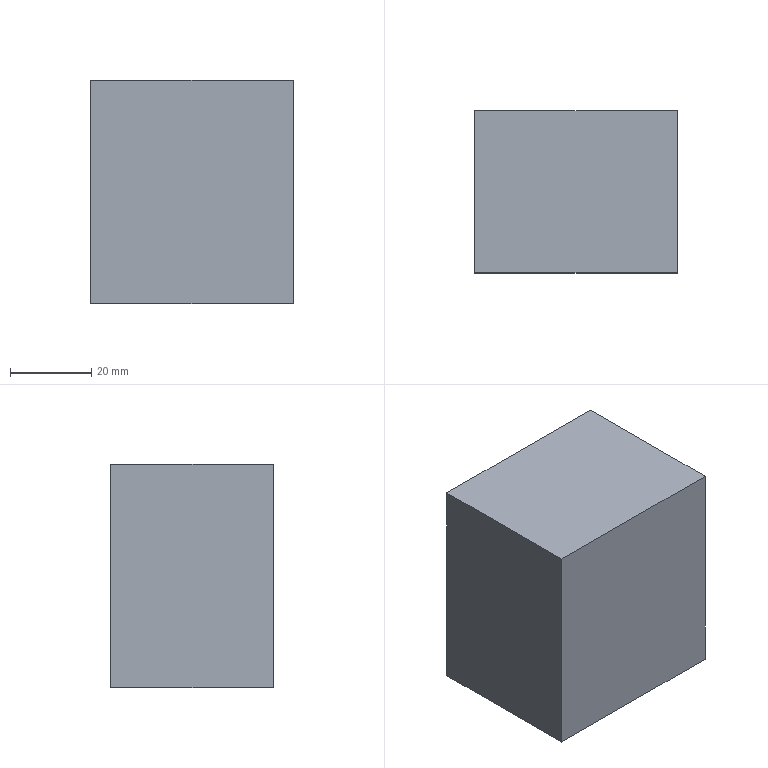Part | NX | features solid 2 | 1 solid | 6 faces | box 50 x 40 x 55.194 mm | volume 110387 mm3 | plane 6
STEP:
#1=CARTESIAN_POINT('',(348.,-205.,10.194));
#2=VERTEX_POINT('',#1);
#3=CARTESIAN_POINT('',(348.,-165.,10.194));
#4=VERTEX_POINT('',#3);
#5=CARTESIAN_POINT('',(348.,-205.,10.194));
#6=DIRECTION('',(0.,-1.,0.));
#7=VECTOR('',#6,1000.);
#8=LINE('',#5,#7);
#9=EDGE_CURVE('',#2,#4,#8,.F.);
#10=ORIENTED_EDGE('',*,*,#9,.T.);
#11=CARTESIAN_POINT('',(298.,-165.,10.194));
#12=VERTEX_POINT('',#11);
#13=CARTESIAN_POINT('',(318.,-165.,10.194));
#14=DIRECTION('',(-1.,0.,0.));
#15=VECTOR('',#14,1000.);
#16=LINE('',#13,#15);
#17=EDGE_CURVE('',#12,#4,#16,.F.);
#18=ORIENTED_EDGE('',*,*,#17,.F.);
#19=CARTESIAN_POINT('',(298.,-205.,10.194));
#20=VERTEX_POINT('',#19);
#21=CARTESIAN_POINT('',(298.,-145.,10.194));
#22=DIRECTION('',(0.,1.,0.));
#23=VECTOR('',#22,1000.);
#24=LINE('',#21,#23);
#25=EDGE_CURVE('',#20,#12,#24,.T.);
#26=ORIENTED_EDGE('',*,*,#25,.F.);
#27=CARTESIAN_POINT('',(323.,-205.,10.194));
#28=DIRECTION('',(-1.,0.,0.));
#29=VECTOR('',#28,1000.);
#30=LINE('',#27,#29);
#31=EDGE_CURVE('',#20,#2,#30,.F.);
#32=ORIENTED_EDGE('',*,*,#31,.T.);
#33=EDGE_LOOP('',(#10,#18,#26,#32));
#34=FACE_BOUND('',#33,.T.);
#35=CARTESIAN_POINT('',(323.,-185.922,10.194));
#36=DIRECTION('',(0.,0.,-1.));
#37=DIRECTION('',(0.9999,0.01247,0.));
#38=AXIS2_PLACEMENT_3D('',#35,#36,#37);
#39=PLANE('',#38);
#40=ADVANCED_FACE('',(#34),#39,.F.);
#41=CARTESIAN_POINT('',(348.,-165.,-45.));
#42=VERTEX_POINT('',#41);
#43=CARTESIAN_POINT('',(348.,-165.,-50.));
#44=DIRECTION('',(0.,0.,1.));
#45=VECTOR('',#44,1000.);
#46=LINE('',#43,#45);
#47=EDGE_CURVE('',#42,#4,#46,.T.);
#48=ORIENTED_EDGE('',*,*,#47,.T.);
#49=ORIENTED_EDGE('',*,*,#9,.F.);
#50=CARTESIAN_POINT('',(348.,-205.,-45.));
#51=VERTEX_POINT('',#50);
#52=CARTESIAN_POINT('',(348.,-205.,-45.));
#53=DIRECTION('',(0.,0.,1.));
#54=VECTOR('',#53,1000.);
#55=LINE('',#52,#54);
#56=EDGE_CURVE('',#51,#2,#55,.T.);
#57=ORIENTED_EDGE('',*,*,#56,.F.);
#58=CARTESIAN_POINT('',(348.,-205.,-45.));
#59=DIRECTION('',(0.,-1.,0.));
#60=VECTOR('',#59,1000.);
#61=LINE('',#58,#60);
#62=EDGE_CURVE('',#51,#42,#61,.F.);
#63=ORIENTED_EDGE('',*,*,#62,.T.);
#64=EDGE_LOOP('',(#48,#49,#57,#63));
#65=FACE_BOUND('',#64,.T.);
#66=CARTESIAN_POINT('',(348.,-205.,-45.));
#67=DIRECTION('',(-1.,0.,0.));
#68=DIRECTION('',(0.,0.,-1.));
#69=AXIS2_PLACEMENT_3D('',#66,#67,#68);
#70=PLANE('',#69);
#71=ADVANCED_FACE('',(#65),#70,.F.);
#72=ORIENTED_EDGE('',*,*,#25,.T.);
#73=CARTESIAN_POINT('',(298.,-165.,-45.));
#74=VERTEX_POINT('',#73);
#75=CARTESIAN_POINT('',(298.,-165.,-50.));
#76=DIRECTION('',(0.,0.,-1.));
#77=VECTOR('',#76,1000.);
#78=LINE('',#75,#77);
#79=EDGE_CURVE('',#74,#12,#78,.F.);
#80=ORIENTED_EDGE('',*,*,#79,.F.);
#81=CARTESIAN_POINT('',(298.,-205.,-45.));
#82=VERTEX_POINT('',#81);
#83=CARTESIAN_POINT('',(298.,-205.,-45.));
#84=DIRECTION('',(0.,1.,0.));
#85=VECTOR('',#84,1000.);
#86=LINE('',#83,#85);
#87=EDGE_CURVE('',#82,#74,#86,.T.);
#88=ORIENTED_EDGE('',*,*,#87,.F.);
#89=CARTESIAN_POINT('',(298.,-205.,-55.));
#90=DIRECTION('',(0.,0.,-1.));
#91=VECTOR('',#90,1000.);
#92=LINE('',#89,#91);
#93=EDGE_CURVE('',#82,#20,#92,.F.);
#94=ORIENTED_EDGE('',*,*,#93,.T.);
#95=EDGE_LOOP('',(#72,#80,#88,#94));
#96=FACE_BOUND('',#95,.T.);
#97=CARTESIAN_POINT('',(298.,-145.,-55.));
#98=DIRECTION('',(1.,0.,0.));
#99=DIRECTION('',(0.,-1.,0.));
#100=AXIS2_PLACEMENT_3D('',#97,#98,#99);
#101=PLANE('',#100);
#102=ADVANCED_FACE('',(#96),#101,.F.);
#103=ORIENTED_EDGE('',*,*,#79,.T.);
#104=ORIENTED_EDGE('',*,*,#17,.T.);
#105=ORIENTED_EDGE('',*,*,#47,.F.);
#106=CARTESIAN_POINT('',(298.,-165.,-45.));
#107=DIRECTION('',(-1.,0.,0.));
#108=VECTOR('',#107,1000.);
#109=LINE('',#106,#108);
#110=EDGE_CURVE('',#74,#42,#109,.F.);
#111=ORIENTED_EDGE('',*,*,#110,.F.);
#112=EDGE_LOOP('',(#103,#104,#105,#111));
#113=FACE_BOUND('',#112,.T.);
#114=CARTESIAN_POINT('',(318.,-165.,-50.));
#115=DIRECTION('',(0.,1.,0.));
#116=DIRECTION('',(1.,0.,0.));
#117=AXIS2_PLACEMENT_3D('',#114,#115,#116);
#118=PLANE('',#117);
#119=ADVANCED_FACE('',(#113),#118,.T.);
#120=ORIENTED_EDGE('',*,*,#62,.F.);
#121=CARTESIAN_POINT('',(298.,-205.,-45.));
#122=DIRECTION('',(1.,0.,0.));
#123=VECTOR('',#122,1000.);
#124=LINE('',#121,#123);
#125=EDGE_CURVE('',#51,#82,#124,.F.);
#126=ORIENTED_EDGE('',*,*,#125,.T.);
#127=ORIENTED_EDGE('',*,*,#87,.T.);
#128=ORIENTED_EDGE('',*,*,#110,.T.);
#129=EDGE_LOOP('',(#120,#126,#127,#128));
#130=FACE_BOUND('',#129,.T.);
#131=CARTESIAN_POINT('',(298.,-205.,-45.));
#132=DIRECTION('',(0.,0.,1.));
#133=DIRECTION('',(0.,1.,0.));
#134=AXIS2_PLACEMENT_3D('',#131,#132,#133);
#135=PLANE('',#134);
#136=ADVANCED_FACE('',(#130),#135,.F.);
#137=ORIENTED_EDGE('',*,*,#125,.F.);
#138=ORIENTED_EDGE('',*,*,#56,.T.);
#139=ORIENTED_EDGE('',*,*,#31,.F.);
#140=ORIENTED_EDGE('',*,*,#93,.F.);
#141=EDGE_LOOP('',(#137,#138,#139,#140));
#142=FACE_BOUND('',#141,.T.);
#143=CARTESIAN_POINT('',(322.5,-205.,-40.721));
#144=DIRECTION('',(0.,-1.,0.));
#145=DIRECTION('',(1.,0.,0.));
#146=AXIS2_PLACEMENT_3D('',#143,#144,#145);
#147=PLANE('',#146);
#148=ADVANCED_FACE('',(#142),#147,.T.);
#149=CLOSED_SHELL('',(#40,#71,#102,#119,#136,#148));
#150=MANIFOLD_SOLID_BREP('',#149);
#151=(LENGTH_UNIT()NAMED_UNIT(*)SI_UNIT(.MILLI.,.METRE.));
#152=UNCERTAINTY_MEASURE_WITH_UNIT(LENGTH_MEASURE(0.00001),#151,'','');
#153=(NAMED_UNIT(*)PLANE_ANGLE_UNIT()SI_UNIT($,.RADIAN.));
#154=(NAMED_UNIT(*)SI_UNIT($,.STERADIAN.)SOLID_ANGLE_UNIT());
#155=(GEOMETRIC_REPRESENTATION_CONTEXT(3)GLOBAL_UNCERTAINTY_ASSIGNED_CONTEXT((#152))GLOBAL_UNIT_ASSIGNED_CONTEXT((#151,#153,#154))REPRESENTATION_CONTEXT('',''));
#156=ADVANCED_BREP_SHAPE_REPRESENTATION('',(#150),#155);